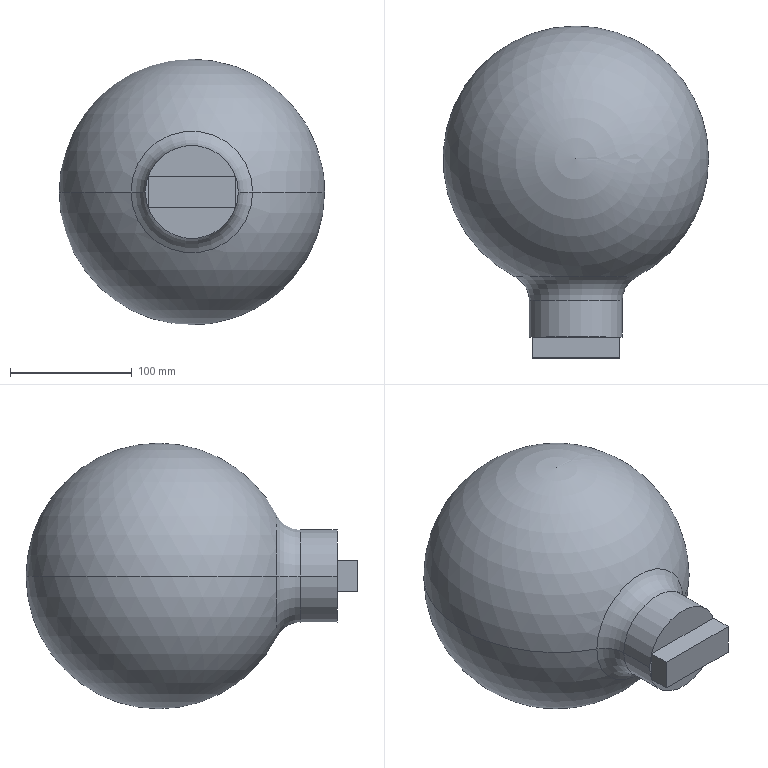Part | SolidWorks | features ICE 4, Revolution 2, Fillet 1, Scale 1 | 2 solids | 13 faces | box 218.44 x 273.05 x 218.44 mm | volume 5685357 mm3 | plane 7 | torus 2 | sphere 2 | cylinder 2 | commonest cylinder face diameters 76.454 x2
STEP:
#1=CARTESIAN_POINT('',(50.059,-97.073,0.));
#2=VERTEX_POINT('',#1);
#3=CARTESIAN_POINT('',(-50.059,-97.073,0.));
#4=VERTEX_POINT('',#3);
#5=CARTESIAN_POINT('',(0.,-97.073,0.));
#6=DIRECTION('',(0.,1.,0.));
#7=DIRECTION('',(-1.,0.,0.));
#8=AXIS2_PLACEMENT_3D('',#5,#6,#7);
#9=CIRCLE('',#8,50.059);
#10=EDGE_CURVE('',#2,#4,#9,.T.);
#11=ORIENTED_EDGE('',*,*,#10,.F.);
#12=CARTESIAN_POINT('',(38.227,-116.487,0.));
#13=VERTEX_POINT('',#12);
#14=CARTESIAN_POINT('',(60.071,-116.487,0.));
#15=DIRECTION('',(0.,0.,1.));
#16=DIRECTION('',(1.,0.,0.));
#17=AXIS2_PLACEMENT_3D('',#14,#15,#16);
#18=CIRCLE('',#17,21.844);
#19=EDGE_CURVE('',#2,#13,#18,.T.);
#20=ORIENTED_EDGE('',*,*,#19,.T.);
#21=CARTESIAN_POINT('',(-38.227,-116.487,0.));
#22=VERTEX_POINT('',#21);
#23=CARTESIAN_POINT('',(0.,-116.487,0.));
#24=DIRECTION('',(0.,-1.,0.));
#25=DIRECTION('',(-1.,0.,0.));
#26=AXIS2_PLACEMENT_3D('',#23,#24,#25);
#27=CIRCLE('',#26,38.227);
#28=EDGE_CURVE('',#22,#13,#27,.T.);
#29=ORIENTED_EDGE('',*,*,#28,.F.);
#30=CARTESIAN_POINT('',(-60.071,-116.487,0.));
#31=DIRECTION('',(0.,0.,-1.));
#32=DIRECTION('',(-1.,0.,0.));
#33=AXIS2_PLACEMENT_3D('',#30,#31,#32);
#34=CIRCLE('',#33,21.844);
#35=EDGE_CURVE('',#4,#22,#34,.T.);
#36=ORIENTED_EDGE('',*,*,#35,.F.);
#37=EDGE_LOOP('',(#11,#20,#29,#36));
#38=FACE_OUTER_BOUND('',#37,.T.);
#39=CARTESIAN_POINT('',(0.,-116.487,0.));
#40=DIRECTION('',(0.,1.,0.));
#41=DIRECTION('',(-1.,0.,0.));
#42=AXIS2_PLACEMENT_3D('',#39,#40,#41);
#43=TOROIDAL_SURFACE('',#42,60.071,21.844);
#44=ADVANCED_FACE('',(#38),#43,.F.);
#45=ORIENTED_EDGE('',*,*,#10,.T.);
#46=CARTESIAN_POINT('',(0.,109.22,0.));
#47=VERTEX_POINT('',#46);
#48=CARTESIAN_POINT('',(0.,0.,0.));
#49=DIRECTION('',(0.,0.,-1.));
#50=DIRECTION('',(-1.,0.,0.));
#51=AXIS2_PLACEMENT_3D('',#48,#49,#50);
#52=CIRCLE('',#51,109.22);
#53=EDGE_CURVE('',#4,#47,#52,.T.);
#54=ORIENTED_EDGE('',*,*,#53,.T.);
#55=CARTESIAN_POINT('',(0.,0.,0.));
#56=DIRECTION('',(0.,0.,1.));
#57=DIRECTION('',(1.,0.,0.));
#58=AXIS2_PLACEMENT_3D('',#55,#56,#57);
#59=CIRCLE('',#58,109.22);
#60=EDGE_CURVE('',#2,#47,#59,.T.);
#61=ORIENTED_EDGE('',*,*,#60,.F.);
#62=EDGE_LOOP('',(#45,#54,#61));
#63=FACE_OUTER_BOUND('',#62,.T.);
#64=CARTESIAN_POINT('',(0.,0.,0.));
#65=DIRECTION('',(0.,0.,-1.));
#66=DIRECTION('',(1.,0.,0.));
#67=AXIS2_PLACEMENT_3D('',#64,#65,#66);
#68=SPHERICAL_SURFACE('',#67,109.22);
#69=ADVANCED_FACE('',(#63),#68,.T.);
#70=CARTESIAN_POINT('',(0.,-116.487,0.));
#71=DIRECTION('',(0.,-1.,0.));
#72=DIRECTION('',(-1.,0.,0.));
#73=AXIS2_PLACEMENT_3D('',#70,#71,#72);
#74=CIRCLE('',#73,38.227);
#75=EDGE_CURVE('',#13,#22,#74,.T.);
#76=ORIENTED_EDGE('',*,*,#75,.T.);
#77=CARTESIAN_POINT('',(-38.227,-146.63,0.));
#78=VERTEX_POINT('',#77);
#79=CARTESIAN_POINT('',(-38.227,-163.83,0.));
#80=DIRECTION('',(0.,-1.,0.));
#81=VECTOR('',#80,1000.);
#82=LINE('',#79,#81);
#83=EDGE_CURVE('',#22,#78,#82,.T.);
#84=ORIENTED_EDGE('',*,*,#83,.T.);
#85=CARTESIAN_POINT('',(38.227,-146.63,0.));
#86=VERTEX_POINT('',#85);
#87=CARTESIAN_POINT('',(0.,-146.63,0.));
#88=DIRECTION('',(0.,1.,0.));
#89=DIRECTION('',(0.,0.,1.));
#90=AXIS2_PLACEMENT_3D('',#87,#88,#89);
#91=CIRCLE('',#90,38.227);
#92=EDGE_CURVE('',#78,#86,#91,.T.);
#93=ORIENTED_EDGE('',*,*,#92,.T.);
#94=CARTESIAN_POINT('',(38.227,-163.83,0.));
#95=DIRECTION('',(0.,-1.,0.));
#96=VECTOR('',#95,1000.);
#97=LINE('',#94,#96);
#98=EDGE_CURVE('',#13,#86,#97,.T.);
#99=ORIENTED_EDGE('',*,*,#98,.F.);
#100=EDGE_LOOP('',(#76,#84,#93,#99));
#101=FACE_OUTER_BOUND('',#100,.T.);
#102=CARTESIAN_POINT('',(0.,-163.83,0.));
#103=DIRECTION('',(0.,-1.,0.));
#104=DIRECTION('',(1.,0.,0.));
#105=AXIS2_PLACEMENT_3D('',#102,#103,#104);
#106=CYLINDRICAL_SURFACE('',#105,38.227);
#107=ADVANCED_FACE('',(#101),#106,.T.);
#108=ORIENTED_EDGE('',*,*,#83,.F.);
#109=ORIENTED_EDGE('',*,*,#28,.T.);
#110=ORIENTED_EDGE('',*,*,#98,.T.);
#111=CARTESIAN_POINT('',(0.,-146.63,0.));
#112=DIRECTION('',(0.,1.,0.));
#113=DIRECTION('',(0.,0.,1.));
#114=AXIS2_PLACEMENT_3D('',#111,#112,#113);
#115=CIRCLE('',#114,38.227);
#116=EDGE_CURVE('',#86,#78,#115,.T.);
#117=ORIENTED_EDGE('',*,*,#116,.T.);
#118=EDGE_LOOP('',(#108,#109,#110,#117));
#119=FACE_OUTER_BOUND('',#118,.T.);
#120=CARTESIAN_POINT('',(0.,-163.83,0.));
#121=DIRECTION('',(0.,-1.,0.));
#122=DIRECTION('',(1.,0.,0.));
#123=AXIS2_PLACEMENT_3D('',#120,#121,#122);
#124=CYLINDRICAL_SURFACE('',#123,38.227);
#125=ADVANCED_FACE('',(#119),#124,.T.);
#126=ORIENTED_EDGE('',*,*,#53,.F.);
#127=CARTESIAN_POINT('',(0.,-97.073,0.));
#128=DIRECTION('',(0.,1.,0.));
#129=DIRECTION('',(-1.,0.,0.));
#130=AXIS2_PLACEMENT_3D('',#127,#128,#129);
#131=CIRCLE('',#130,50.059);
#132=EDGE_CURVE('',#4,#2,#131,.T.);
#133=ORIENTED_EDGE('',*,*,#132,.T.);
#134=ORIENTED_EDGE('',*,*,#60,.T.);
#135=EDGE_LOOP('',(#126,#133,#134));
#136=FACE_OUTER_BOUND('',#135,.T.);
#137=CARTESIAN_POINT('',(0.,0.,0.));
#138=DIRECTION('',(0.,0.,-1.));
#139=DIRECTION('',(1.,0.,0.));
#140=AXIS2_PLACEMENT_3D('',#137,#138,#139);
#141=SPHERICAL_SURFACE('',#140,109.22);
#142=ADVANCED_FACE('',(#136),#141,.T.);
#143=ORIENTED_EDGE('',*,*,#19,.F.);
#144=ORIENTED_EDGE('',*,*,#132,.F.);
#145=ORIENTED_EDGE('',*,*,#35,.T.);
#146=ORIENTED_EDGE('',*,*,#75,.F.);
#147=EDGE_LOOP('',(#143,#144,#145,#146));
#148=FACE_OUTER_BOUND('',#147,.T.);
#149=CARTESIAN_POINT('',(0.,-116.487,0.));
#150=DIRECTION('',(0.,1.,0.));
#151=DIRECTION('',(-1.,0.,0.));
#152=AXIS2_PLACEMENT_3D('',#149,#150,#151);
#153=TOROIDAL_SURFACE('',#152,60.071,21.844);
#154=ADVANCED_FACE('',(#148),#153,.F.);
#155=ORIENTED_EDGE('',*,*,#116,.F.);
#156=ORIENTED_EDGE('',*,*,#92,.F.);
#157=EDGE_LOOP('',(#155,#156));
#158=FACE_OUTER_BOUND('',#157,.T.);
#159=CARTESIAN_POINT('',(-109.22,-146.63,68.001));
#160=DIRECTION('',(0.,1.,0.));
#161=DIRECTION('',(0.,0.,1.));
#162=AXIS2_PLACEMENT_3D('',#159,#160,#161);
#163=PLANE('',#162);
#164=ADVANCED_FACE('',(#158),#163,.F.);
#165=CLOSED_SHELL('',(#44,#69,#107,#125,#142,#154,#164));
#166=MANIFOLD_SOLID_BREP('',#165);
#167=CARTESIAN_POINT('',(-35.985,-146.63,12.9));
#168=VERTEX_POINT('',#167);
#169=CARTESIAN_POINT('',(-35.985,-146.63,-12.9));
#170=VERTEX_POINT('',#169);
#171=CARTESIAN_POINT('',(-35.985,-146.63,-12.9));
#172=DIRECTION('',(0.,0.,-1.));
#173=VECTOR('',#172,1000.);
#174=LINE('',#171,#173);
#175=EDGE_CURVE('',#168,#170,#174,.T.);
#176=ORIENTED_EDGE('',*,*,#175,.T.);
#177=CARTESIAN_POINT('',(-35.985,-163.83,-12.9));
#178=VERTEX_POINT('',#177);
#179=CARTESIAN_POINT('',(-35.985,-163.83,-12.9));
#180=DIRECTION('',(0.,1.,0.));
#181=VECTOR('',#180,1000.);
#182=LINE('',#179,#181);
#183=EDGE_CURVE('',#178,#170,#182,.T.);
#184=ORIENTED_EDGE('',*,*,#183,.F.);
#185=CARTESIAN_POINT('',(-35.985,-163.83,12.9));
#186=VERTEX_POINT('',#185);
#187=CARTESIAN_POINT('',(-35.985,-163.83,-12.9));
#188=DIRECTION('',(0.,0.,-1.));
#189=VECTOR('',#188,1000.);
#190=LINE('',#187,#189);
#191=EDGE_CURVE('',#186,#178,#190,.T.);
#192=ORIENTED_EDGE('',*,*,#191,.F.);
#193=CARTESIAN_POINT('',(-35.985,-163.83,12.9));
#194=DIRECTION('',(0.,1.,0.));
#195=VECTOR('',#194,1000.);
#196=LINE('',#193,#195);
#197=EDGE_CURVE('',#186,#168,#196,.T.);
#198=ORIENTED_EDGE('',*,*,#197,.T.);
#199=EDGE_LOOP('',(#176,#184,#192,#198));
#200=FACE_OUTER_BOUND('',#199,.T.);
#201=CARTESIAN_POINT('',(-35.985,-163.83,-12.9));
#202=DIRECTION('',(1.,0.,0.));
#203=DIRECTION('',(0.,0.,-1.));
#204=AXIS2_PLACEMENT_3D('',#201,#202,#203);
#205=PLANE('',#204);
#206=ADVANCED_FACE('',(#200),#205,.F.);
#207=CARTESIAN_POINT('',(35.985,-146.63,-12.9));
#208=VERTEX_POINT('',#207);
#209=CARTESIAN_POINT('',(35.985,-146.63,-12.9));
#210=DIRECTION('',(1.,0.,0.));
#211=VECTOR('',#210,1000.);
#212=LINE('',#209,#211);
#213=EDGE_CURVE('',#170,#208,#212,.T.);
#214=ORIENTED_EDGE('',*,*,#213,.T.);
#215=CARTESIAN_POINT('',(35.985,-163.83,-12.9));
#216=VERTEX_POINT('',#215);
#217=CARTESIAN_POINT('',(35.985,-163.83,-12.9));
#218=DIRECTION('',(0.,1.,0.));
#219=VECTOR('',#218,1000.);
#220=LINE('',#217,#219);
#221=EDGE_CURVE('',#216,#208,#220,.T.);
#222=ORIENTED_EDGE('',*,*,#221,.F.);
#223=CARTESIAN_POINT('',(35.985,-163.83,-12.9));
#224=DIRECTION('',(1.,0.,0.));
#225=VECTOR('',#224,1000.);
#226=LINE('',#223,#225);
#227=EDGE_CURVE('',#178,#216,#226,.T.);
#228=ORIENTED_EDGE('',*,*,#227,.F.);
#229=ORIENTED_EDGE('',*,*,#183,.T.);
#230=EDGE_LOOP('',(#214,#222,#228,#229));
#231=FACE_OUTER_BOUND('',#230,.T.);
#232=CARTESIAN_POINT('',(35.985,-163.83,-12.9));
#233=DIRECTION('',(0.,0.,1.));
#234=DIRECTION('',(1.,0.,0.));
#235=AXIS2_PLACEMENT_3D('',#232,#233,#234);
#236=PLANE('',#235);
#237=ADVANCED_FACE('',(#231),#236,.F.);
#238=CARTESIAN_POINT('',(35.985,-146.63,12.9));
#239=VERTEX_POINT('',#238);
#240=CARTESIAN_POINT('',(35.985,-146.63,-12.9));
#241=DIRECTION('',(0.,0.,1.));
#242=VECTOR('',#241,1000.);
#243=LINE('',#240,#242);
#244=EDGE_CURVE('',#208,#239,#243,.T.);
#245=ORIENTED_EDGE('',*,*,#244,.T.);
#246=CARTESIAN_POINT('',(35.985,-163.83,12.9));
#247=VERTEX_POINT('',#246);
#248=CARTESIAN_POINT('',(35.985,-163.83,12.9));
#249=DIRECTION('',(0.,1.,0.));
#250=VECTOR('',#249,1000.);
#251=LINE('',#248,#250);
#252=EDGE_CURVE('',#247,#239,#251,.T.);
#253=ORIENTED_EDGE('',*,*,#252,.F.);
#254=CARTESIAN_POINT('',(35.985,-163.83,-12.9));
#255=DIRECTION('',(0.,0.,1.));
#256=VECTOR('',#255,1000.);
#257=LINE('',#254,#256);
#258=EDGE_CURVE('',#216,#247,#257,.T.);
#259=ORIENTED_EDGE('',*,*,#258,.F.);
#260=ORIENTED_EDGE('',*,*,#221,.T.);
#261=EDGE_LOOP('',(#245,#253,#259,#260));
#262=FACE_OUTER_BOUND('',#261,.T.);
#263=CARTESIAN_POINT('',(35.985,-163.83,-12.9));
#264=DIRECTION('',(-1.,0.,0.));
#265=DIRECTION('',(0.,0.,1.));
#266=AXIS2_PLACEMENT_3D('',#263,#264,#265);
#267=PLANE('',#266);
#268=ADVANCED_FACE('',(#262),#267,.F.);
#269=CARTESIAN_POINT('',(35.985,-146.63,12.9));
#270=DIRECTION('',(-1.,0.,0.));
#271=VECTOR('',#270,1000.);
#272=LINE('',#269,#271);
#273=EDGE_CURVE('',#239,#168,#272,.T.);
#274=ORIENTED_EDGE('',*,*,#273,.T.);
#275=ORIENTED_EDGE('',*,*,#197,.F.);
#276=CARTESIAN_POINT('',(35.985,-163.83,12.9));
#277=DIRECTION('',(-1.,0.,0.));
#278=VECTOR('',#277,1000.);
#279=LINE('',#276,#278);
#280=EDGE_CURVE('',#247,#186,#279,.T.);
#281=ORIENTED_EDGE('',*,*,#280,.F.);
#282=ORIENTED_EDGE('',*,*,#252,.T.);
#283=EDGE_LOOP('',(#274,#275,#281,#282));
#284=FACE_OUTER_BOUND('',#283,.T.);
#285=CARTESIAN_POINT('',(35.985,-163.83,12.9));
#286=DIRECTION('',(0.,0.,-1.));
#287=DIRECTION('',(-1.,0.,0.));
#288=AXIS2_PLACEMENT_3D('',#285,#286,#287);
#289=PLANE('',#288);
#290=ADVANCED_FACE('',(#284),#289,.F.);
#291=ORIENTED_EDGE('',*,*,#191,.T.);
#292=ORIENTED_EDGE('',*,*,#227,.T.);
#293=ORIENTED_EDGE('',*,*,#258,.T.);
#294=ORIENTED_EDGE('',*,*,#280,.T.);
#295=EDGE_LOOP('',(#291,#292,#293,#294));
#296=FACE_OUTER_BOUND('',#295,.T.);
#297=CARTESIAN_POINT('',(0.,-163.83,0.));
#298=DIRECTION('',(0.,-1.,0.));
#299=DIRECTION('',(0.,0.,-1.));
#300=AXIS2_PLACEMENT_3D('',#297,#298,#299);
#301=PLANE('',#300);
#302=ADVANCED_FACE('',(#296),#301,.T.);
#303=ORIENTED_EDGE('',*,*,#175,.F.);
#304=ORIENTED_EDGE('',*,*,#273,.F.);
#305=ORIENTED_EDGE('',*,*,#244,.F.);
#306=ORIENTED_EDGE('',*,*,#213,.F.);
#307=EDGE_LOOP('',(#303,#304,#305,#306));
#308=FACE_OUTER_BOUND('',#307,.T.);
#309=CARTESIAN_POINT('',(0.,-146.63,0.));
#310=DIRECTION('',(0.,-1.,0.));
#311=DIRECTION('',(0.,0.,-1.));
#312=AXIS2_PLACEMENT_3D('',#309,#310,#311);
#313=PLANE('',#312);
#314=ADVANCED_FACE('',(#308),#313,.F.);
#315=CLOSED_SHELL('',(#206,#237,#268,#290,#302,#314));
#316=MANIFOLD_SOLID_BREP('',#315);
#317=CARTESIAN_POINT('',(0.,0.,0.));
#318=DIRECTION('',(0.,0.,1.));
#319=DIRECTION('',(1.,0.,0.));
#320=AXIS2_PLACEMENT_3D('',#317,#318,#319);
#321=(LENGTH_UNIT()NAMED_UNIT(*)SI_UNIT(.MILLI.,.METRE.));
#322=UNCERTAINTY_MEASURE_WITH_UNIT(LENGTH_MEASURE(0.00001),#321,'','');
#323=(NAMED_UNIT(*)PLANE_ANGLE_UNIT()SI_UNIT($,.RADIAN.));
#324=(NAMED_UNIT(*)SI_UNIT($,.STERADIAN.)SOLID_ANGLE_UNIT());
#325=(GEOMETRIC_REPRESENTATION_CONTEXT(3)GLOBAL_UNCERTAINTY_ASSIGNED_CONTEXT((#322))GLOBAL_UNIT_ASSIGNED_CONTEXT((#321,#323,#324))REPRESENTATION_CONTEXT('',''));
#326=ADVANCED_BREP_SHAPE_REPRESENTATION('',(#166,#316,#320),#325);